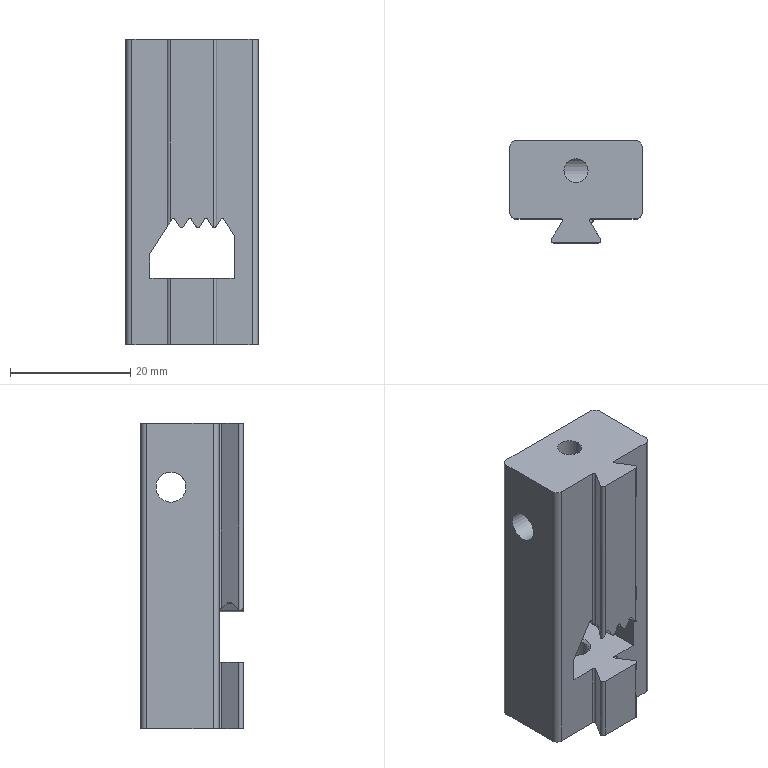Part | STEP file | 1 solid | 54 faces | box 22 x 17 x 50.8 mm | volume 13297 mm3 | plane 28 | cylinder 24 | cone 2 | commonest cylinder face diameters 0.62 x6 0.78 x4 1 x4 2 x4 0.6 x3 4.01 x1